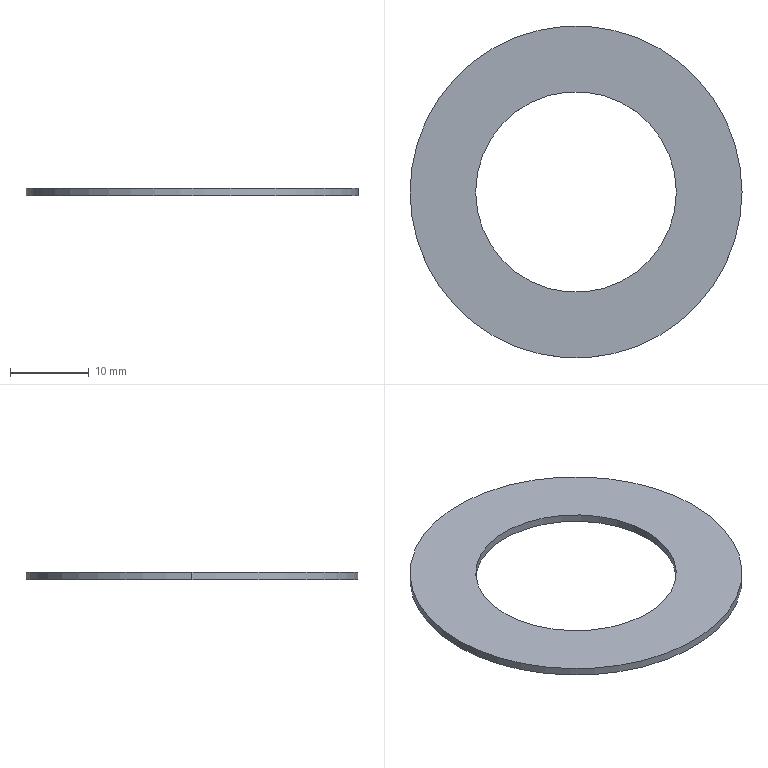Part | NX | features BREP 1 | 1 solid | 6 faces | box 42.2 x 42.2 x 1 mm | volume 887.963 mm3 | cylinder 4 | plane 2 | commonest cylinder face diameters 25.5 x2 42.2 x2
STEP:
#1=CARTESIAN_POINT('',(-287.044,27.798,1.));
#2=VERTEX_POINT('',#1);
#3=CARTESIAN_POINT('',(-261.544,27.798,1.));
#4=VERTEX_POINT('',#3);
#5=CARTESIAN_POINT('',(-274.294,27.798,1.));
#6=DIRECTION('',(0.,0.,1.));
#7=DIRECTION('',(1.,0.,0.));
#8=AXIS2_PLACEMENT_3D('',#5,#6,#7);
#9=CIRCLE('',#8,12.75);
#10=EDGE_CURVE('',#2,#4,#9,.T.);
#11=ORIENTED_EDGE('',*,*,#10,.T.);
#12=CARTESIAN_POINT('',(-261.544,27.798,0.));
#13=VERTEX_POINT('',#12);
#14=CARTESIAN_POINT('',(-261.544,27.798,1.5));
#15=DIRECTION('',(0.,0.,-1.));
#16=VECTOR('',#15,1000.);
#17=LINE('',#14,#16);
#18=EDGE_CURVE('',#13,#4,#17,.F.);
#19=ORIENTED_EDGE('',*,*,#18,.F.);
#20=CARTESIAN_POINT('',(-287.044,27.798,0.));
#21=VERTEX_POINT('',#20);
#22=CARTESIAN_POINT('',(-274.294,27.798,0.));
#23=DIRECTION('',(0.,0.,1.));
#24=DIRECTION('',(1.,0.,0.));
#25=AXIS2_PLACEMENT_3D('',#22,#23,#24);
#26=CIRCLE('',#25,12.75);
#27=EDGE_CURVE('',#21,#13,#26,.T.);
#28=ORIENTED_EDGE('',*,*,#27,.F.);
#29=CARTESIAN_POINT('',(-287.044,27.798,1.5));
#30=DIRECTION('',(0.,0.,-1.));
#31=VECTOR('',#30,1000.);
#32=LINE('',#29,#31);
#33=EDGE_CURVE('',#21,#2,#32,.F.);
#34=ORIENTED_EDGE('',*,*,#33,.T.);
#35=EDGE_LOOP('',(#11,#19,#28,#34));
#36=FACE_BOUND('',#35,.T.);
#37=CARTESIAN_POINT('',(-274.294,27.798,1.5));
#38=DIRECTION('',(0.,0.,-1.));
#39=DIRECTION('',(1.,0.,0.));
#40=AXIS2_PLACEMENT_3D('',#37,#38,#39);
#41=CYLINDRICAL_SURFACE('',#40,12.75);
#42=ADVANCED_FACE('',(#36),#41,.F.);
#43=CARTESIAN_POINT('',(-253.194,27.798,1.));
#44=VERTEX_POINT('',#43);
#45=CARTESIAN_POINT('',(-295.394,27.798,1.));
#46=VERTEX_POINT('',#45);
#47=CARTESIAN_POINT('',(-274.294,27.798,1.));
#48=DIRECTION('',(0.,0.,1.));
#49=DIRECTION('',(1.,0.,0.));
#50=AXIS2_PLACEMENT_3D('',#47,#48,#49);
#51=CIRCLE('',#50,21.1);
#52=EDGE_CURVE('',#44,#46,#51,.T.);
#53=ORIENTED_EDGE('',*,*,#52,.F.);
#54=CARTESIAN_POINT('',(-253.194,27.798,0.));
#55=VERTEX_POINT('',#54);
#56=CARTESIAN_POINT('',(-253.194,27.798,1.5));
#57=DIRECTION('',(0.,0.,-1.));
#58=VECTOR('',#57,1000.);
#59=LINE('',#56,#58);
#60=EDGE_CURVE('',#55,#44,#59,.F.);
#61=ORIENTED_EDGE('',*,*,#60,.F.);
#62=CARTESIAN_POINT('',(-295.394,27.798,0.));
#63=VERTEX_POINT('',#62);
#64=CARTESIAN_POINT('',(-274.294,27.798,0.));
#65=DIRECTION('',(0.,0.,1.));
#66=DIRECTION('',(1.,0.,0.));
#67=AXIS2_PLACEMENT_3D('',#64,#65,#66);
#68=CIRCLE('',#67,21.1);
#69=EDGE_CURVE('',#55,#63,#68,.T.);
#70=ORIENTED_EDGE('',*,*,#69,.T.);
#71=CARTESIAN_POINT('',(-295.394,27.798,1.5));
#72=DIRECTION('',(0.,0.,-1.));
#73=VECTOR('',#72,1000.);
#74=LINE('',#71,#73);
#75=EDGE_CURVE('',#63,#46,#74,.F.);
#76=ORIENTED_EDGE('',*,*,#75,.T.);
#77=EDGE_LOOP('',(#53,#61,#70,#76));
#78=FACE_BOUND('',#77,.T.);
#79=CARTESIAN_POINT('',(-274.294,27.798,1.5));
#80=DIRECTION('',(0.,0.,-1.));
#81=DIRECTION('',(1.,0.,0.));
#82=AXIS2_PLACEMENT_3D('',#79,#80,#81);
#83=CYLINDRICAL_SURFACE('',#82,21.1);
#84=ADVANCED_FACE('',(#78),#83,.T.);
#85=CARTESIAN_POINT('',(-274.294,27.798,1.));
#86=DIRECTION('',(0.,0.,1.));
#87=DIRECTION('',(1.,0.,0.));
#88=AXIS2_PLACEMENT_3D('',#85,#86,#87);
#89=CIRCLE('',#88,21.1);
#90=EDGE_CURVE('',#46,#44,#89,.T.);
#91=ORIENTED_EDGE('',*,*,#90,.T.);
#92=ORIENTED_EDGE('',*,*,#52,.T.);
#93=EDGE_LOOP('',(#91,#92));
#94=FACE_BOUND('',#93,.T.);
#95=ORIENTED_EDGE('',*,*,#10,.F.);
#96=CARTESIAN_POINT('',(-274.294,27.798,1.));
#97=DIRECTION('',(0.,0.,1.));
#98=DIRECTION('',(1.,0.,0.));
#99=AXIS2_PLACEMENT_3D('',#96,#97,#98);
#100=CIRCLE('',#99,12.75);
#101=EDGE_CURVE('',#4,#2,#100,.T.);
#102=ORIENTED_EDGE('',*,*,#101,.F.);
#103=EDGE_LOOP('',(#95,#102));
#104=FACE_BOUND('',#103,.T.);
#105=CARTESIAN_POINT('',(-274.294,27.798,1.));
#106=DIRECTION('',(0.,0.,1.));
#107=DIRECTION('',(-1.,0.,0.));
#108=AXIS2_PLACEMENT_3D('',#105,#106,#107);
#109=PLANE('',#108);
#110=ADVANCED_FACE('',(#94,#104),#109,.T.);
#111=CARTESIAN_POINT('',(-274.294,27.798,0.));
#112=DIRECTION('',(0.,0.,1.));
#113=DIRECTION('',(1.,0.,0.));
#114=AXIS2_PLACEMENT_3D('',#111,#112,#113);
#115=CIRCLE('',#114,21.1);
#116=EDGE_CURVE('',#63,#55,#115,.T.);
#117=ORIENTED_EDGE('',*,*,#116,.F.);
#118=ORIENTED_EDGE('',*,*,#69,.F.);
#119=EDGE_LOOP('',(#117,#118));
#120=FACE_BOUND('',#119,.T.);
#121=ORIENTED_EDGE('',*,*,#27,.T.);
#122=CARTESIAN_POINT('',(-274.294,27.798,0.));
#123=DIRECTION('',(0.,0.,1.));
#124=DIRECTION('',(1.,0.,0.));
#125=AXIS2_PLACEMENT_3D('',#122,#123,#124);
#126=CIRCLE('',#125,12.75);
#127=EDGE_CURVE('',#13,#21,#126,.T.);
#128=ORIENTED_EDGE('',*,*,#127,.T.);
#129=EDGE_LOOP('',(#121,#128));
#130=FACE_BOUND('',#129,.T.);
#131=CARTESIAN_POINT('',(-274.294,27.798,0.));
#132=DIRECTION('',(0.,0.,1.));
#133=DIRECTION('',(-1.,0.,0.));
#134=AXIS2_PLACEMENT_3D('',#131,#132,#133);
#135=PLANE('',#134);
#136=ADVANCED_FACE('',(#120,#130),#135,.F.);
#137=ORIENTED_EDGE('',*,*,#60,.T.);
#138=ORIENTED_EDGE('',*,*,#90,.F.);
#139=ORIENTED_EDGE('',*,*,#75,.F.);
#140=ORIENTED_EDGE('',*,*,#116,.T.);
#141=EDGE_LOOP('',(#137,#138,#139,#140));
#142=FACE_BOUND('',#141,.T.);
#143=CARTESIAN_POINT('',(-274.294,27.798,1.5));
#144=DIRECTION('',(0.,0.,-1.));
#145=DIRECTION('',(1.,0.,0.));
#146=AXIS2_PLACEMENT_3D('',#143,#144,#145);
#147=CYLINDRICAL_SURFACE('',#146,21.1);
#148=ADVANCED_FACE('',(#142),#147,.T.);
#149=ORIENTED_EDGE('',*,*,#18,.T.);
#150=ORIENTED_EDGE('',*,*,#101,.T.);
#151=ORIENTED_EDGE('',*,*,#33,.F.);
#152=ORIENTED_EDGE('',*,*,#127,.F.);
#153=EDGE_LOOP('',(#149,#150,#151,#152));
#154=FACE_BOUND('',#153,.T.);
#155=CARTESIAN_POINT('',(-274.294,27.798,1.5));
#156=DIRECTION('',(0.,0.,-1.));
#157=DIRECTION('',(1.,0.,0.));
#158=AXIS2_PLACEMENT_3D('',#155,#156,#157);
#159=CYLINDRICAL_SURFACE('',#158,12.75);
#160=ADVANCED_FACE('',(#154),#159,.F.);
#161=CLOSED_SHELL('',(#42,#84,#110,#136,#148,#160));
#162=MANIFOLD_SOLID_BREP('',#161);
#163=(LENGTH_UNIT()NAMED_UNIT(*)SI_UNIT(.MILLI.,.METRE.));
#164=UNCERTAINTY_MEASURE_WITH_UNIT(LENGTH_MEASURE(0.00001),#163,'','');
#165=(NAMED_UNIT(*)PLANE_ANGLE_UNIT()SI_UNIT($,.RADIAN.));
#166=(NAMED_UNIT(*)SI_UNIT($,.STERADIAN.)SOLID_ANGLE_UNIT());
#167=(GEOMETRIC_REPRESENTATION_CONTEXT(3)GLOBAL_UNCERTAINTY_ASSIGNED_CONTEXT((#164))GLOBAL_UNIT_ASSIGNED_CONTEXT((#163,#165,#166))REPRESENTATION_CONTEXT('',''));
#168=ADVANCED_BREP_SHAPE_REPRESENTATION('',(#162),#167);